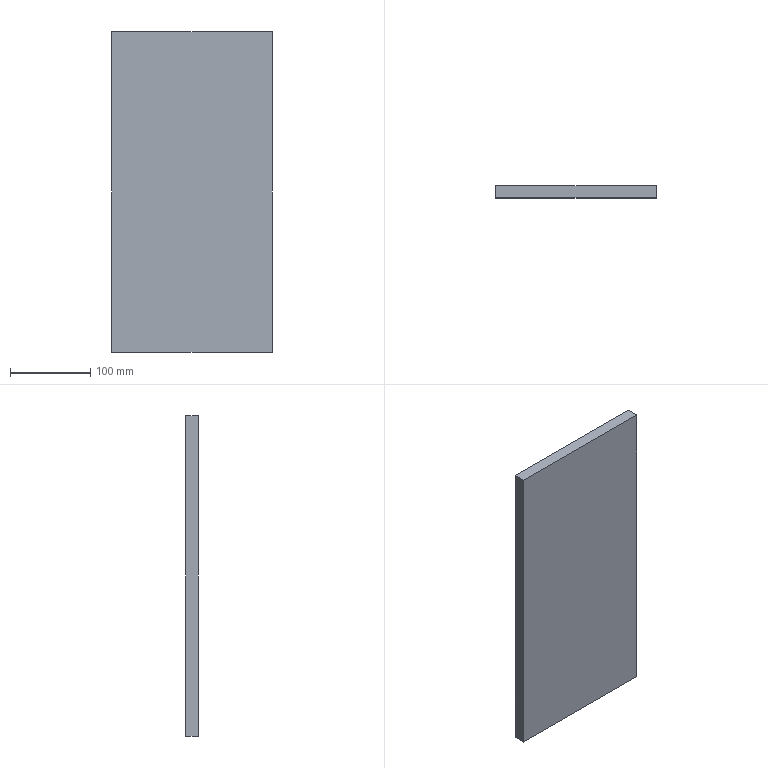Part | SolidWorks | features Extrusion 1, HoleWzd 1 | 1 solid | 22 faces | box 200 x 15 x 400 mm | volume 1194970 mm3 | cylinder 8 | cone 8 | plane 6 | commonest cylinder face diameters 20 x8
STEP:
#1=CARTESIAN_POINT('',(-75.,13.,-160.));
#2=VERTEX_POINT('',#1);
#3=CARTESIAN_POINT('',(-75.,13.,-140.));
#4=VERTEX_POINT('',#3);
#5=CARTESIAN_POINT('',(-75.,13.,-150.));
#6=DIRECTION('',(0.,1.,0.));
#7=DIRECTION('',(0.,0.,1.));
#8=AXIS2_PLACEMENT_3D('',#5,#6,#7);
#9=CIRCLE('',#8,10.);
#10=EDGE_CURVE('',#2,#4,#9,.T.);
#11=ORIENTED_EDGE('',*,*,#10,.F.);
#12=CARTESIAN_POINT('',(-75.,15.,-160.));
#13=VERTEX_POINT('',#12);
#14=CARTESIAN_POINT('',(-75.,15.,-160.));
#15=DIRECTION('',(0.,1.,0.));
#16=VECTOR('',#15,1000.);
#17=LINE('',#14,#16);
#18=EDGE_CURVE('',#2,#13,#17,.T.);
#19=ORIENTED_EDGE('',*,*,#18,.T.);
#20=CARTESIAN_POINT('',(-75.,15.,-140.));
#21=VERTEX_POINT('',#20);
#22=CARTESIAN_POINT('',(-75.,15.,-150.));
#23=DIRECTION('',(0.,1.,0.));
#24=DIRECTION('',(0.,0.,1.));
#25=AXIS2_PLACEMENT_3D('',#22,#23,#24);
#26=CIRCLE('',#25,10.);
#27=EDGE_CURVE('',#13,#21,#26,.T.);
#28=ORIENTED_EDGE('',*,*,#27,.T.);
#29=CARTESIAN_POINT('',(-75.,15.,-140.));
#30=DIRECTION('',(0.,1.,0.));
#31=VECTOR('',#30,1000.);
#32=LINE('',#29,#31);
#33=EDGE_CURVE('',#4,#21,#32,.T.);
#34=ORIENTED_EDGE('',*,*,#33,.F.);
#35=EDGE_LOOP('',(#11,#19,#28,#34));
#36=FACE_OUTER_BOUND('',#35,.T.);
#37=CARTESIAN_POINT('',(-75.,15.,-150.));
#38=DIRECTION('',(0.,1.,0.));
#39=DIRECTION('',(0.,0.,1.));
#40=AXIS2_PLACEMENT_3D('',#37,#38,#39);
#41=CYLINDRICAL_SURFACE('',#40,10.);
#42=ADVANCED_FACE('',(#36),#41,.F.);
#43=CARTESIAN_POINT('',(-75.,6.991,-150.));
#44=VERTEX_POINT('',#43);
#45=CARTESIAN_POINT('',(-75.,13.,-140.));
#46=DIRECTION('',(0.,0.515,0.8572));
#47=VECTOR('',#46,1000.);
#48=LINE('',#45,#47);
#49=EDGE_CURVE('',#44,#4,#48,.T.);
#50=ORIENTED_EDGE('',*,*,#49,.F.);
#51=CARTESIAN_POINT('',(-75.,13.,-160.));
#52=DIRECTION('',(0.,0.515,-0.8572));
#53=VECTOR('',#52,1000.);
#54=LINE('',#51,#53);
#55=EDGE_CURVE('',#44,#2,#54,.T.);
#56=ORIENTED_EDGE('',*,*,#55,.T.);
#57=ORIENTED_EDGE('',*,*,#10,.T.);
#58=EDGE_LOOP('',(#50,#56,#57));
#59=FACE_OUTER_BOUND('',#58,.T.);
#60=CARTESIAN_POINT('',(-75.,13.,-150.));
#61=DIRECTION('',(0.,1.,0.));
#62=DIRECTION('',(0.,0.,1.));
#63=AXIS2_PLACEMENT_3D('',#60,#61,#62);
#64=CONICAL_SURFACE('',#63,10.,1.03);
#65=ADVANCED_FACE('',(#59),#64,.F.);
#66=CARTESIAN_POINT('',(-75.,13.,140.));
#67=VERTEX_POINT('',#66);
#68=CARTESIAN_POINT('',(-75.,13.,160.));
#69=VERTEX_POINT('',#68);
#70=CARTESIAN_POINT('',(-75.,13.,150.));
#71=DIRECTION('',(0.,1.,0.));
#72=DIRECTION('',(0.,0.,1.));
#73=AXIS2_PLACEMENT_3D('',#70,#71,#72);
#74=CIRCLE('',#73,10.);
#75=EDGE_CURVE('',#67,#69,#74,.T.);
#76=ORIENTED_EDGE('',*,*,#75,.F.);
#77=CARTESIAN_POINT('',(-75.,15.,140.));
#78=VERTEX_POINT('',#77);
#79=CARTESIAN_POINT('',(-75.,15.,140.));
#80=DIRECTION('',(0.,1.,0.));
#81=VECTOR('',#80,1000.);
#82=LINE('',#79,#81);
#83=EDGE_CURVE('',#67,#78,#82,.T.);
#84=ORIENTED_EDGE('',*,*,#83,.T.);
#85=CARTESIAN_POINT('',(-75.,15.,160.));
#86=VERTEX_POINT('',#85);
#87=CARTESIAN_POINT('',(-75.,15.,150.));
#88=DIRECTION('',(0.,1.,0.));
#89=DIRECTION('',(0.,0.,1.));
#90=AXIS2_PLACEMENT_3D('',#87,#88,#89);
#91=CIRCLE('',#90,10.);
#92=EDGE_CURVE('',#78,#86,#91,.T.);
#93=ORIENTED_EDGE('',*,*,#92,.T.);
#94=CARTESIAN_POINT('',(-75.,15.,160.));
#95=DIRECTION('',(0.,1.,0.));
#96=VECTOR('',#95,1000.);
#97=LINE('',#94,#96);
#98=EDGE_CURVE('',#69,#86,#97,.T.);
#99=ORIENTED_EDGE('',*,*,#98,.F.);
#100=EDGE_LOOP('',(#76,#84,#93,#99));
#101=FACE_OUTER_BOUND('',#100,.T.);
#102=CARTESIAN_POINT('',(-75.,15.,150.));
#103=DIRECTION('',(0.,1.,0.));
#104=DIRECTION('',(0.,0.,1.));
#105=AXIS2_PLACEMENT_3D('',#102,#103,#104);
#106=CYLINDRICAL_SURFACE('',#105,10.);
#107=ADVANCED_FACE('',(#101),#106,.F.);
#108=CARTESIAN_POINT('',(-75.,6.991,150.));
#109=VERTEX_POINT('',#108);
#110=CARTESIAN_POINT('',(-75.,13.,160.));
#111=DIRECTION('',(0.,0.515,0.8572));
#112=VECTOR('',#111,1000.);
#113=LINE('',#110,#112);
#114=EDGE_CURVE('',#109,#69,#113,.T.);
#115=ORIENTED_EDGE('',*,*,#114,.F.);
#116=CARTESIAN_POINT('',(-75.,13.,140.));
#117=DIRECTION('',(0.,0.515,-0.8572));
#118=VECTOR('',#117,1000.);
#119=LINE('',#116,#118);
#120=EDGE_CURVE('',#109,#67,#119,.T.);
#121=ORIENTED_EDGE('',*,*,#120,.T.);
#122=ORIENTED_EDGE('',*,*,#75,.T.);
#123=EDGE_LOOP('',(#115,#121,#122));
#124=FACE_OUTER_BOUND('',#123,.T.);
#125=CARTESIAN_POINT('',(-75.,13.,150.));
#126=DIRECTION('',(0.,1.,0.));
#127=DIRECTION('',(0.,0.,1.));
#128=AXIS2_PLACEMENT_3D('',#125,#126,#127);
#129=CONICAL_SURFACE('',#128,10.,1.03);
#130=ADVANCED_FACE('',(#124),#129,.F.);
#131=CARTESIAN_POINT('',(75.,13.,140.));
#132=VERTEX_POINT('',#131);
#133=CARTESIAN_POINT('',(75.,13.,160.));
#134=VERTEX_POINT('',#133);
#135=CARTESIAN_POINT('',(75.,13.,150.));
#136=DIRECTION('',(0.,1.,0.));
#137=DIRECTION('',(0.,0.,1.));
#138=AXIS2_PLACEMENT_3D('',#135,#136,#137);
#139=CIRCLE('',#138,10.);
#140=EDGE_CURVE('',#132,#134,#139,.T.);
#141=ORIENTED_EDGE('',*,*,#140,.F.);
#142=CARTESIAN_POINT('',(75.,15.,140.));
#143=VERTEX_POINT('',#142);
#144=CARTESIAN_POINT('',(75.,15.,140.));
#145=DIRECTION('',(0.,1.,0.));
#146=VECTOR('',#145,1000.);
#147=LINE('',#144,#146);
#148=EDGE_CURVE('',#132,#143,#147,.T.);
#149=ORIENTED_EDGE('',*,*,#148,.T.);
#150=CARTESIAN_POINT('',(75.,15.,160.));
#151=VERTEX_POINT('',#150);
#152=CARTESIAN_POINT('',(75.,15.,150.));
#153=DIRECTION('',(0.,1.,0.));
#154=DIRECTION('',(0.,0.,1.));
#155=AXIS2_PLACEMENT_3D('',#152,#153,#154);
#156=CIRCLE('',#155,10.);
#157=EDGE_CURVE('',#143,#151,#156,.T.);
#158=ORIENTED_EDGE('',*,*,#157,.T.);
#159=CARTESIAN_POINT('',(75.,15.,160.));
#160=DIRECTION('',(0.,1.,0.));
#161=VECTOR('',#160,1000.);
#162=LINE('',#159,#161);
#163=EDGE_CURVE('',#134,#151,#162,.T.);
#164=ORIENTED_EDGE('',*,*,#163,.F.);
#165=EDGE_LOOP('',(#141,#149,#158,#164));
#166=FACE_OUTER_BOUND('',#165,.T.);
#167=CARTESIAN_POINT('',(75.,15.,150.));
#168=DIRECTION('',(0.,1.,0.));
#169=DIRECTION('',(0.,0.,1.));
#170=AXIS2_PLACEMENT_3D('',#167,#168,#169);
#171=CYLINDRICAL_SURFACE('',#170,10.);
#172=ADVANCED_FACE('',(#166),#171,.F.);
#173=CARTESIAN_POINT('',(75.,6.991,150.));
#174=VERTEX_POINT('',#173);
#175=CARTESIAN_POINT('',(75.,13.,160.));
#176=DIRECTION('',(0.,0.515,0.8572));
#177=VECTOR('',#176,1000.);
#178=LINE('',#175,#177);
#179=EDGE_CURVE('',#174,#134,#178,.T.);
#180=ORIENTED_EDGE('',*,*,#179,.F.);
#181=CARTESIAN_POINT('',(75.,13.,140.));
#182=DIRECTION('',(0.,0.515,-0.8572));
#183=VECTOR('',#182,1000.);
#184=LINE('',#181,#183);
#185=EDGE_CURVE('',#174,#132,#184,.T.);
#186=ORIENTED_EDGE('',*,*,#185,.T.);
#187=ORIENTED_EDGE('',*,*,#140,.T.);
#188=EDGE_LOOP('',(#180,#186,#187));
#189=FACE_OUTER_BOUND('',#188,.T.);
#190=CARTESIAN_POINT('',(75.,13.,150.));
#191=DIRECTION('',(0.,1.,0.));
#192=DIRECTION('',(0.,0.,1.));
#193=AXIS2_PLACEMENT_3D('',#190,#191,#192);
#194=CONICAL_SURFACE('',#193,10.,1.03);
#195=ADVANCED_FACE('',(#189),#194,.F.);
#196=CARTESIAN_POINT('',(75.,13.,-160.));
#197=VERTEX_POINT('',#196);
#198=CARTESIAN_POINT('',(75.,13.,-140.));
#199=VERTEX_POINT('',#198);
#200=CARTESIAN_POINT('',(75.,13.,-150.));
#201=DIRECTION('',(0.,1.,0.));
#202=DIRECTION('',(0.,0.,1.));
#203=AXIS2_PLACEMENT_3D('',#200,#201,#202);
#204=CIRCLE('',#203,10.);
#205=EDGE_CURVE('',#197,#199,#204,.T.);
#206=ORIENTED_EDGE('',*,*,#205,.F.);
#207=CARTESIAN_POINT('',(75.,15.,-160.));
#208=VERTEX_POINT('',#207);
#209=CARTESIAN_POINT('',(75.,15.,-160.));
#210=DIRECTION('',(0.,1.,0.));
#211=VECTOR('',#210,1000.);
#212=LINE('',#209,#211);
#213=EDGE_CURVE('',#197,#208,#212,.T.);
#214=ORIENTED_EDGE('',*,*,#213,.T.);
#215=CARTESIAN_POINT('',(75.,15.,-140.));
#216=VERTEX_POINT('',#215);
#217=CARTESIAN_POINT('',(75.,15.,-150.));
#218=DIRECTION('',(0.,1.,0.));
#219=DIRECTION('',(0.,0.,1.));
#220=AXIS2_PLACEMENT_3D('',#217,#218,#219);
#221=CIRCLE('',#220,10.);
#222=EDGE_CURVE('',#208,#216,#221,.T.);
#223=ORIENTED_EDGE('',*,*,#222,.T.);
#224=CARTESIAN_POINT('',(75.,15.,-140.));
#225=DIRECTION('',(0.,1.,0.));
#226=VECTOR('',#225,1000.);
#227=LINE('',#224,#226);
#228=EDGE_CURVE('',#199,#216,#227,.T.);
#229=ORIENTED_EDGE('',*,*,#228,.F.);
#230=EDGE_LOOP('',(#206,#214,#223,#229));
#231=FACE_OUTER_BOUND('',#230,.T.);
#232=CARTESIAN_POINT('',(75.,15.,-150.));
#233=DIRECTION('',(0.,1.,0.));
#234=DIRECTION('',(0.,0.,1.));
#235=AXIS2_PLACEMENT_3D('',#232,#233,#234);
#236=CYLINDRICAL_SURFACE('',#235,10.);
#237=ADVANCED_FACE('',(#231),#236,.F.);
#238=CARTESIAN_POINT('',(75.,6.991,-150.));
#239=VERTEX_POINT('',#238);
#240=CARTESIAN_POINT('',(75.,13.,-140.));
#241=DIRECTION('',(0.,0.515,0.8572));
#242=VECTOR('',#241,1000.);
#243=LINE('',#240,#242);
#244=EDGE_CURVE('',#239,#199,#243,.T.);
#245=ORIENTED_EDGE('',*,*,#244,.F.);
#246=CARTESIAN_POINT('',(75.,13.,-160.));
#247=DIRECTION('',(0.,0.515,-0.8572));
#248=VECTOR('',#247,1000.);
#249=LINE('',#246,#248);
#250=EDGE_CURVE('',#239,#197,#249,.T.);
#251=ORIENTED_EDGE('',*,*,#250,.T.);
#252=ORIENTED_EDGE('',*,*,#205,.T.);
#253=EDGE_LOOP('',(#245,#251,#252));
#254=FACE_OUTER_BOUND('',#253,.T.);
#255=CARTESIAN_POINT('',(75.,13.,-150.));
#256=DIRECTION('',(0.,1.,0.));
#257=DIRECTION('',(0.,0.,1.));
#258=AXIS2_PLACEMENT_3D('',#255,#256,#257);
#259=CONICAL_SURFACE('',#258,10.,1.03);
#260=ADVANCED_FACE('',(#254),#259,.F.);
#261=CARTESIAN_POINT('',(100.,0.,200.));
#262=VERTEX_POINT('',#261);
#263=CARTESIAN_POINT('',(100.,0.,-200.));
#264=VERTEX_POINT('',#263);
#265=CARTESIAN_POINT('',(100.,0.,-200.));
#266=DIRECTION('',(0.,0.,-1.));
#267=VECTOR('',#266,1000.);
#268=LINE('',#265,#267);
#269=EDGE_CURVE('',#262,#264,#268,.T.);
#270=ORIENTED_EDGE('',*,*,#269,.T.);
#271=CARTESIAN_POINT('',(100.,15.,-200.));
#272=VERTEX_POINT('',#271);
#273=CARTESIAN_POINT('',(100.,15.,-200.));
#274=DIRECTION('',(0.,-1.,0.));
#275=VECTOR('',#274,1000.);
#276=LINE('',#273,#275);
#277=EDGE_CURVE('',#272,#264,#276,.T.);
#278=ORIENTED_EDGE('',*,*,#277,.F.);
#279=CARTESIAN_POINT('',(100.,15.,200.));
#280=VERTEX_POINT('',#279);
#281=CARTESIAN_POINT('',(100.,15.,-200.));
#282=DIRECTION('',(0.,0.,-1.));
#283=VECTOR('',#282,1000.);
#284=LINE('',#281,#283);
#285=EDGE_CURVE('',#280,#272,#284,.T.);
#286=ORIENTED_EDGE('',*,*,#285,.F.);
#287=CARTESIAN_POINT('',(100.,15.,200.));
#288=DIRECTION('',(0.,-1.,0.));
#289=VECTOR('',#288,1000.);
#290=LINE('',#287,#289);
#291=EDGE_CURVE('',#280,#262,#290,.T.);
#292=ORIENTED_EDGE('',*,*,#291,.T.);
#293=EDGE_LOOP('',(#270,#278,#286,#292));
#294=FACE_OUTER_BOUND('',#293,.T.);
#295=CARTESIAN_POINT('',(100.,15.,-200.));
#296=DIRECTION('',(-1.,0.,0.));
#297=DIRECTION('',(0.,0.,1.));
#298=AXIS2_PLACEMENT_3D('',#295,#296,#297);
#299=PLANE('',#298);
#300=ADVANCED_FACE('',(#294),#299,.F.);
#301=CARTESIAN_POINT('',(-100.,0.,-200.));
#302=VERTEX_POINT('',#301);
#303=CARTESIAN_POINT('',(-100.,0.,-200.));
#304=DIRECTION('',(-1.,0.,0.));
#305=VECTOR('',#304,1000.);
#306=LINE('',#303,#305);
#307=EDGE_CURVE('',#264,#302,#306,.T.);
#308=ORIENTED_EDGE('',*,*,#307,.T.);
#309=CARTESIAN_POINT('',(-100.,15.,-200.));
#310=VERTEX_POINT('',#309);
#311=CARTESIAN_POINT('',(-100.,15.,-200.));
#312=DIRECTION('',(0.,-1.,0.));
#313=VECTOR('',#312,1000.);
#314=LINE('',#311,#313);
#315=EDGE_CURVE('',#310,#302,#314,.T.);
#316=ORIENTED_EDGE('',*,*,#315,.F.);
#317=CARTESIAN_POINT('',(-100.,15.,-200.));
#318=DIRECTION('',(-1.,0.,0.));
#319=VECTOR('',#318,1000.);
#320=LINE('',#317,#319);
#321=EDGE_CURVE('',#272,#310,#320,.T.);
#322=ORIENTED_EDGE('',*,*,#321,.F.);
#323=ORIENTED_EDGE('',*,*,#277,.T.);
#324=EDGE_LOOP('',(#308,#316,#322,#323));
#325=FACE_OUTER_BOUND('',#324,.T.);
#326=CARTESIAN_POINT('',(-100.,15.,-200.));
#327=DIRECTION('',(0.,0.,1.));
#328=DIRECTION('',(1.,0.,0.));
#329=AXIS2_PLACEMENT_3D('',#326,#327,#328);
#330=PLANE('',#329);
#331=ADVANCED_FACE('',(#325),#330,.F.);
#332=CARTESIAN_POINT('',(-100.,0.,200.));
#333=VERTEX_POINT('',#332);
#334=CARTESIAN_POINT('',(-100.,0.,-200.));
#335=DIRECTION('',(0.,0.,1.));
#336=VECTOR('',#335,1000.);
#337=LINE('',#334,#336);
#338=EDGE_CURVE('',#302,#333,#337,.T.);
#339=ORIENTED_EDGE('',*,*,#338,.T.);
#340=CARTESIAN_POINT('',(-100.,15.,200.));
#341=VERTEX_POINT('',#340);
#342=CARTESIAN_POINT('',(-100.,15.,200.));
#343=DIRECTION('',(0.,-1.,0.));
#344=VECTOR('',#343,1000.);
#345=LINE('',#342,#344);
#346=EDGE_CURVE('',#341,#333,#345,.T.);
#347=ORIENTED_EDGE('',*,*,#346,.F.);
#348=CARTESIAN_POINT('',(-100.,15.,-200.));
#349=DIRECTION('',(0.,0.,1.));
#350=VECTOR('',#349,1000.);
#351=LINE('',#348,#350);
#352=EDGE_CURVE('',#310,#341,#351,.T.);
#353=ORIENTED_EDGE('',*,*,#352,.F.);
#354=ORIENTED_EDGE('',*,*,#315,.T.);
#355=EDGE_LOOP('',(#339,#347,#353,#354));
#356=FACE_OUTER_BOUND('',#355,.T.);
#357=CARTESIAN_POINT('',(-100.,15.,-200.));
#358=DIRECTION('',(1.,0.,0.));
#359=DIRECTION('',(0.,0.,-1.));
#360=AXIS2_PLACEMENT_3D('',#357,#358,#359);
#361=PLANE('',#360);
#362=ADVANCED_FACE('',(#356),#361,.F.);
#363=CARTESIAN_POINT('',(-100.,0.,200.));
#364=DIRECTION('',(1.,0.,0.));
#365=VECTOR('',#364,1000.);
#366=LINE('',#363,#365);
#367=EDGE_CURVE('',#333,#262,#366,.T.);
#368=ORIENTED_EDGE('',*,*,#367,.T.);
#369=ORIENTED_EDGE('',*,*,#291,.F.);
#370=CARTESIAN_POINT('',(-100.,15.,200.));
#371=DIRECTION('',(1.,0.,0.));
#372=VECTOR('',#371,1000.);
#373=LINE('',#370,#372);
#374=EDGE_CURVE('',#341,#280,#373,.T.);
#375=ORIENTED_EDGE('',*,*,#374,.F.);
#376=ORIENTED_EDGE('',*,*,#346,.T.);
#377=EDGE_LOOP('',(#368,#369,#375,#376));
#378=FACE_OUTER_BOUND('',#377,.T.);
#379=CARTESIAN_POINT('',(-100.,15.,200.));
#380=DIRECTION('',(0.,0.,-1.));
#381=DIRECTION('',(-1.,0.,0.));
#382=AXIS2_PLACEMENT_3D('',#379,#380,#381);
#383=PLANE('',#382);
#384=ADVANCED_FACE('',(#378),#383,.F.);
#385=CARTESIAN_POINT('',(-75.,15.,-150.));
#386=DIRECTION('',(0.,1.,0.));
#387=DIRECTION('',(0.,0.,1.));
#388=AXIS2_PLACEMENT_3D('',#385,#386,#387);
#389=CIRCLE('',#388,10.);
#390=EDGE_CURVE('',#21,#13,#389,.T.);
#391=ORIENTED_EDGE('',*,*,#390,.F.);
#392=ORIENTED_EDGE('',*,*,#27,.F.);
#393=EDGE_LOOP('',(#391,#392));
#394=FACE_BOUND('',#393,.T.);
#395=CARTESIAN_POINT('',(-75.,15.,150.));
#396=DIRECTION('',(0.,1.,0.));
#397=DIRECTION('',(0.,0.,1.));
#398=AXIS2_PLACEMENT_3D('',#395,#396,#397);
#399=CIRCLE('',#398,10.);
#400=EDGE_CURVE('',#86,#78,#399,.T.);
#401=ORIENTED_EDGE('',*,*,#400,.F.);
#402=ORIENTED_EDGE('',*,*,#92,.F.);
#403=EDGE_LOOP('',(#401,#402));
#404=FACE_BOUND('',#403,.T.);
#405=CARTESIAN_POINT('',(75.,15.,150.));
#406=DIRECTION('',(0.,1.,0.));
#407=DIRECTION('',(0.,0.,1.));
#408=AXIS2_PLACEMENT_3D('',#405,#406,#407);
#409=CIRCLE('',#408,10.);
#410=EDGE_CURVE('',#151,#143,#409,.T.);
#411=ORIENTED_EDGE('',*,*,#410,.F.);
#412=ORIENTED_EDGE('',*,*,#157,.F.);
#413=EDGE_LOOP('',(#411,#412));
#414=FACE_BOUND('',#413,.T.);
#415=CARTESIAN_POINT('',(75.,15.,-150.));
#416=DIRECTION('',(0.,1.,0.));
#417=DIRECTION('',(0.,0.,1.));
#418=AXIS2_PLACEMENT_3D('',#415,#416,#417);
#419=CIRCLE('',#418,10.);
#420=EDGE_CURVE('',#216,#208,#419,.T.);
#421=ORIENTED_EDGE('',*,*,#420,.F.);
#422=ORIENTED_EDGE('',*,*,#222,.F.);
#423=EDGE_LOOP('',(#421,#422));
#424=FACE_BOUND('',#423,.T.);
#425=ORIENTED_EDGE('',*,*,#285,.T.);
#426=ORIENTED_EDGE('',*,*,#321,.T.);
#427=ORIENTED_EDGE('',*,*,#352,.T.);
#428=ORIENTED_EDGE('',*,*,#374,.T.);
#429=EDGE_LOOP('',(#425,#426,#427,#428));
#430=FACE_OUTER_BOUND('',#429,.T.);
#431=CARTESIAN_POINT('',(0.,15.,0.));
#432=DIRECTION('',(0.,1.,0.));
#433=DIRECTION('',(0.,0.,1.));
#434=AXIS2_PLACEMENT_3D('',#431,#432,#433);
#435=PLANE('',#434);
#436=ADVANCED_FACE('',(#394,#404,#414,#424,#430),#435,.T.);
#437=ORIENTED_EDGE('',*,*,#269,.F.);
#438=ORIENTED_EDGE('',*,*,#367,.F.);
#439=ORIENTED_EDGE('',*,*,#338,.F.);
#440=ORIENTED_EDGE('',*,*,#307,.F.);
#441=EDGE_LOOP('',(#437,#438,#439,#440));
#442=FACE_OUTER_BOUND('',#441,.T.);
#443=CARTESIAN_POINT('',(0.,0.,0.));
#444=DIRECTION('',(0.,1.,0.));
#445=DIRECTION('',(0.,0.,1.));
#446=AXIS2_PLACEMENT_3D('',#443,#444,#445);
#447=PLANE('',#446);
#448=ADVANCED_FACE('',(#442),#447,.F.);
#449=ORIENTED_EDGE('',*,*,#250,.F.);
#450=ORIENTED_EDGE('',*,*,#244,.T.);
#451=CARTESIAN_POINT('',(75.,13.,-150.));
#452=DIRECTION('',(0.,1.,0.));
#453=DIRECTION('',(0.,0.,1.));
#454=AXIS2_PLACEMENT_3D('',#451,#452,#453);
#455=CIRCLE('',#454,10.);
#456=EDGE_CURVE('',#199,#197,#455,.T.);
#457=ORIENTED_EDGE('',*,*,#456,.T.);
#458=EDGE_LOOP('',(#449,#450,#457));
#459=FACE_OUTER_BOUND('',#458,.T.);
#460=CARTESIAN_POINT('',(75.,13.,-150.));
#461=DIRECTION('',(0.,1.,0.));
#462=DIRECTION('',(0.,0.,1.));
#463=AXIS2_PLACEMENT_3D('',#460,#461,#462);
#464=CONICAL_SURFACE('',#463,10.,1.03);
#465=ADVANCED_FACE('',(#459),#464,.F.);
#466=ORIENTED_EDGE('',*,*,#213,.F.);
#467=ORIENTED_EDGE('',*,*,#456,.F.);
#468=ORIENTED_EDGE('',*,*,#228,.T.);
#469=ORIENTED_EDGE('',*,*,#420,.T.);
#470=EDGE_LOOP('',(#466,#467,#468,#469));
#471=FACE_OUTER_BOUND('',#470,.T.);
#472=CARTESIAN_POINT('',(75.,15.,-150.));
#473=DIRECTION('',(0.,1.,0.));
#474=DIRECTION('',(0.,0.,1.));
#475=AXIS2_PLACEMENT_3D('',#472,#473,#474);
#476=CYLINDRICAL_SURFACE('',#475,10.);
#477=ADVANCED_FACE('',(#471),#476,.F.);
#478=ORIENTED_EDGE('',*,*,#185,.F.);
#479=ORIENTED_EDGE('',*,*,#179,.T.);
#480=CARTESIAN_POINT('',(75.,13.,150.));
#481=DIRECTION('',(0.,1.,0.));
#482=DIRECTION('',(0.,0.,1.));
#483=AXIS2_PLACEMENT_3D('',#480,#481,#482);
#484=CIRCLE('',#483,10.);
#485=EDGE_CURVE('',#134,#132,#484,.T.);
#486=ORIENTED_EDGE('',*,*,#485,.T.);
#487=EDGE_LOOP('',(#478,#479,#486));
#488=FACE_OUTER_BOUND('',#487,.T.);
#489=CARTESIAN_POINT('',(75.,13.,150.));
#490=DIRECTION('',(0.,1.,0.));
#491=DIRECTION('',(0.,0.,1.));
#492=AXIS2_PLACEMENT_3D('',#489,#490,#491);
#493=CONICAL_SURFACE('',#492,10.,1.03);
#494=ADVANCED_FACE('',(#488),#493,.F.);
#495=ORIENTED_EDGE('',*,*,#148,.F.);
#496=ORIENTED_EDGE('',*,*,#485,.F.);
#497=ORIENTED_EDGE('',*,*,#163,.T.);
#498=ORIENTED_EDGE('',*,*,#410,.T.);
#499=EDGE_LOOP('',(#495,#496,#497,#498));
#500=FACE_OUTER_BOUND('',#499,.T.);
#501=CARTESIAN_POINT('',(75.,15.,150.));
#502=DIRECTION('',(0.,1.,0.));
#503=DIRECTION('',(0.,0.,1.));
#504=AXIS2_PLACEMENT_3D('',#501,#502,#503);
#505=CYLINDRICAL_SURFACE('',#504,10.);
#506=ADVANCED_FACE('',(#500),#505,.F.);
#507=ORIENTED_EDGE('',*,*,#120,.F.);
#508=ORIENTED_EDGE('',*,*,#114,.T.);
#509=CARTESIAN_POINT('',(-75.,13.,150.));
#510=DIRECTION('',(0.,1.,0.));
#511=DIRECTION('',(0.,0.,1.));
#512=AXIS2_PLACEMENT_3D('',#509,#510,#511);
#513=CIRCLE('',#512,10.);
#514=EDGE_CURVE('',#69,#67,#513,.T.);
#515=ORIENTED_EDGE('',*,*,#514,.T.);
#516=EDGE_LOOP('',(#507,#508,#515));
#517=FACE_OUTER_BOUND('',#516,.T.);
#518=CARTESIAN_POINT('',(-75.,13.,150.));
#519=DIRECTION('',(0.,1.,0.));
#520=DIRECTION('',(0.,0.,1.));
#521=AXIS2_PLACEMENT_3D('',#518,#519,#520);
#522=CONICAL_SURFACE('',#521,10.,1.03);
#523=ADVANCED_FACE('',(#517),#522,.F.);
#524=ORIENTED_EDGE('',*,*,#83,.F.);
#525=ORIENTED_EDGE('',*,*,#514,.F.);
#526=ORIENTED_EDGE('',*,*,#98,.T.);
#527=ORIENTED_EDGE('',*,*,#400,.T.);
#528=EDGE_LOOP('',(#524,#525,#526,#527));
#529=FACE_OUTER_BOUND('',#528,.T.);
#530=CARTESIAN_POINT('',(-75.,15.,150.));
#531=DIRECTION('',(0.,1.,0.));
#532=DIRECTION('',(0.,0.,1.));
#533=AXIS2_PLACEMENT_3D('',#530,#531,#532);
#534=CYLINDRICAL_SURFACE('',#533,10.);
#535=ADVANCED_FACE('',(#529),#534,.F.);
#536=ORIENTED_EDGE('',*,*,#55,.F.);
#537=ORIENTED_EDGE('',*,*,#49,.T.);
#538=CARTESIAN_POINT('',(-75.,13.,-150.));
#539=DIRECTION('',(0.,1.,0.));
#540=DIRECTION('',(0.,0.,1.));
#541=AXIS2_PLACEMENT_3D('',#538,#539,#540);
#542=CIRCLE('',#541,10.);
#543=EDGE_CURVE('',#4,#2,#542,.T.);
#544=ORIENTED_EDGE('',*,*,#543,.T.);
#545=EDGE_LOOP('',(#536,#537,#544));
#546=FACE_OUTER_BOUND('',#545,.T.);
#547=CARTESIAN_POINT('',(-75.,13.,-150.));
#548=DIRECTION('',(0.,1.,0.));
#549=DIRECTION('',(0.,0.,1.));
#550=AXIS2_PLACEMENT_3D('',#547,#548,#549);
#551=CONICAL_SURFACE('',#550,10.,1.03);
#552=ADVANCED_FACE('',(#546),#551,.F.);
#553=ORIENTED_EDGE('',*,*,#18,.F.);
#554=ORIENTED_EDGE('',*,*,#543,.F.);
#555=ORIENTED_EDGE('',*,*,#33,.T.);
#556=ORIENTED_EDGE('',*,*,#390,.T.);
#557=EDGE_LOOP('',(#553,#554,#555,#556));
#558=FACE_OUTER_BOUND('',#557,.T.);
#559=CARTESIAN_POINT('',(-75.,15.,-150.));
#560=DIRECTION('',(0.,1.,0.));
#561=DIRECTION('',(0.,0.,1.));
#562=AXIS2_PLACEMENT_3D('',#559,#560,#561);
#563=CYLINDRICAL_SURFACE('',#562,10.);
#564=ADVANCED_FACE('',(#558),#563,.F.);
#565=CLOSED_SHELL('',(#42,#65,#107,#130,#172,#195,#237,#260,#300,#331,#362,#384,#436,#448,#465,#477,#494,#506,#523,#535,#552,#564));
#566=MANIFOLD_SOLID_BREP('',#565);
#567=CARTESIAN_POINT('',(0.,0.,0.));
#568=DIRECTION('',(0.,0.,1.));
#569=DIRECTION('',(1.,0.,0.));
#570=AXIS2_PLACEMENT_3D('',#567,#568,#569);
#571=(LENGTH_UNIT()NAMED_UNIT(*)SI_UNIT(.MILLI.,.METRE.));
#572=UNCERTAINTY_MEASURE_WITH_UNIT(LENGTH_MEASURE(0.00001),#571,'','');
#573=(NAMED_UNIT(*)PLANE_ANGLE_UNIT()SI_UNIT($,.RADIAN.));
#574=(NAMED_UNIT(*)SI_UNIT($,.STERADIAN.)SOLID_ANGLE_UNIT());
#575=(GEOMETRIC_REPRESENTATION_CONTEXT(3)GLOBAL_UNCERTAINTY_ASSIGNED_CONTEXT((#572))GLOBAL_UNIT_ASSIGNED_CONTEXT((#571,#573,#574))REPRESENTATION_CONTEXT('',''));
#576=ADVANCED_BREP_SHAPE_REPRESENTATION('',(#566,#570),#575);